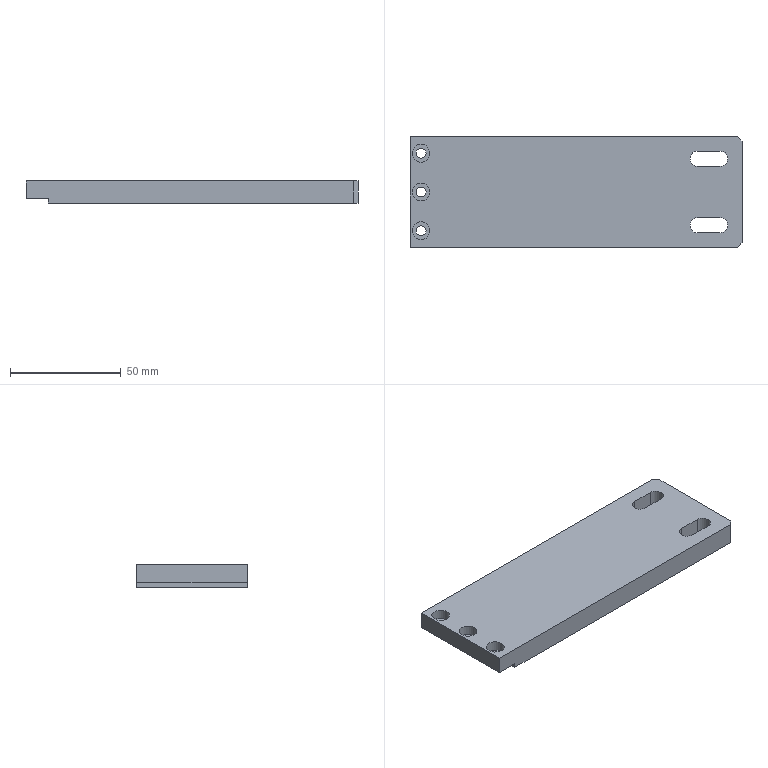Part | NX | 1 solid | 27 faces | box 150 x 50 x 10 mm | volume 70934 mm3 | plane 17 | cylinder 10 | commonest cylinder face diameters 7 x4 4.5 x3 8 x3
STEP:
#1=CARTESIAN_POINT('',(-75.,-25.,2.));
#2=VERTEX_POINT('',#1);
#3=CARTESIAN_POINT('',(-75.,25.,2.));
#4=VERTEX_POINT('',#3);
#5=CARTESIAN_POINT('',(-75.,-25.,2.));
#6=DIRECTION('',(0.,1.,0.));
#7=VECTOR('',#6,1000.);
#8=LINE('',#5,#7);
#9=EDGE_CURVE('',#2,#4,#8,.T.);
#10=ORIENTED_EDGE('',*,*,#9,.F.);
#11=CARTESIAN_POINT('',(-75.,-25.,10.));
#12=VERTEX_POINT('',#11);
#13=CARTESIAN_POINT('',(-75.,-25.,10.));
#14=DIRECTION('',(0.,0.,-1.));
#15=VECTOR('',#14,1000.);
#16=LINE('',#13,#15);
#17=EDGE_CURVE('',#12,#2,#16,.T.);
#18=ORIENTED_EDGE('',*,*,#17,.F.);
#19=CARTESIAN_POINT('',(-75.,25.,10.));
#20=VERTEX_POINT('',#19);
#21=CARTESIAN_POINT('',(-75.,-25.,10.));
#22=DIRECTION('',(0.,-1.,0.));
#23=VECTOR('',#22,1000.);
#24=LINE('',#21,#23);
#25=EDGE_CURVE('',#20,#12,#24,.T.);
#26=ORIENTED_EDGE('',*,*,#25,.F.);
#27=CARTESIAN_POINT('',(-75.,25.,10.));
#28=DIRECTION('',(0.,0.,-1.));
#29=VECTOR('',#28,1000.);
#30=LINE('',#27,#29);
#31=EDGE_CURVE('',#20,#4,#30,.T.);
#32=ORIENTED_EDGE('',*,*,#31,.T.);
#33=EDGE_LOOP('',(#10,#18,#26,#32));
#34=FACE_BOUND('',#33,.T.);
#35=CARTESIAN_POINT('',(-75.,-25.,10.));
#36=DIRECTION('',(1.,0.,0.));
#37=DIRECTION('',(0.,0.,-1.));
#38=AXIS2_PLACEMENT_3D('',#35,#36,#37);
#39=PLANE('',#38);
#40=ADVANCED_FACE('',(#34),#39,.F.);
#41=CARTESIAN_POINT('',(-67.75,-17.5,5.4));
#42=VERTEX_POINT('',#41);
#43=CARTESIAN_POINT('',(-70.,-17.5,5.4));
#44=DIRECTION('',(0.,0.,1.));
#45=DIRECTION('',(1.,0.,0.));
#46=AXIS2_PLACEMENT_3D('',#43,#44,#45);
#47=CIRCLE('',#46,2.25);
#48=EDGE_CURVE('',#42,#42,#47,.T.);
#49=ORIENTED_EDGE('',*,*,#48,.T.);
#50=EDGE_LOOP('',(#49));
#51=FACE_BOUND('',#50,.T.);
#52=CARTESIAN_POINT('',(-72.25,-17.5,2.));
#53=VERTEX_POINT('',#52);
#54=CARTESIAN_POINT('',(-70.,-17.5,2.));
#55=DIRECTION('',(0.,0.,-1.));
#56=DIRECTION('',(-1.,0.,0.));
#57=AXIS2_PLACEMENT_3D('',#54,#55,#56);
#58=CIRCLE('',#57,2.25);
#59=EDGE_CURVE('',#53,#53,#58,.F.);
#60=ORIENTED_EDGE('',*,*,#59,.F.);
#61=EDGE_LOOP('',(#60));
#62=FACE_BOUND('',#61,.T.);
#63=CARTESIAN_POINT('',(-70.,-17.5,10.));
#64=DIRECTION('',(0.,0.,1.));
#65=DIRECTION('',(1.,0.,0.));
#66=AXIS2_PLACEMENT_3D('',#63,#64,#65);
#67=CYLINDRICAL_SURFACE('',#66,2.25);
#68=ADVANCED_FACE('',(#51,#62),#67,.F.);
#69=CARTESIAN_POINT('',(-67.75,0.,5.4));
#70=VERTEX_POINT('',#69);
#71=CARTESIAN_POINT('',(-70.,0.,5.4));
#72=DIRECTION('',(0.,0.,1.));
#73=DIRECTION('',(1.,0.,0.));
#74=AXIS2_PLACEMENT_3D('',#71,#72,#73);
#75=CIRCLE('',#74,2.25);
#76=EDGE_CURVE('',#70,#70,#75,.T.);
#77=ORIENTED_EDGE('',*,*,#76,.T.);
#78=EDGE_LOOP('',(#77));
#79=FACE_BOUND('',#78,.T.);
#80=CARTESIAN_POINT('',(-72.25,0.,2.));
#81=VERTEX_POINT('',#80);
#82=CARTESIAN_POINT('',(-70.,0.,2.));
#83=DIRECTION('',(0.,0.,-1.));
#84=DIRECTION('',(-1.,0.,0.));
#85=AXIS2_PLACEMENT_3D('',#82,#83,#84);
#86=CIRCLE('',#85,2.25);
#87=EDGE_CURVE('',#81,#81,#86,.F.);
#88=ORIENTED_EDGE('',*,*,#87,.F.);
#89=EDGE_LOOP('',(#88));
#90=FACE_BOUND('',#89,.T.);
#91=CARTESIAN_POINT('',(-70.,0.,10.));
#92=DIRECTION('',(0.,0.,1.));
#93=DIRECTION('',(1.,0.,0.));
#94=AXIS2_PLACEMENT_3D('',#91,#92,#93);
#95=CYLINDRICAL_SURFACE('',#94,2.25);
#96=ADVANCED_FACE('',(#79,#90),#95,.F.);
#97=CARTESIAN_POINT('',(-67.75,17.5,5.4));
#98=VERTEX_POINT('',#97);
#99=CARTESIAN_POINT('',(-70.,17.5,5.4));
#100=DIRECTION('',(0.,0.,1.));
#101=DIRECTION('',(1.,0.,0.));
#102=AXIS2_PLACEMENT_3D('',#99,#100,#101);
#103=CIRCLE('',#102,2.25);
#104=EDGE_CURVE('',#98,#98,#103,.T.);
#105=ORIENTED_EDGE('',*,*,#104,.T.);
#106=EDGE_LOOP('',(#105));
#107=FACE_BOUND('',#106,.T.);
#108=CARTESIAN_POINT('',(-72.25,17.5,2.));
#109=VERTEX_POINT('',#108);
#110=CARTESIAN_POINT('',(-70.,17.5,2.));
#111=DIRECTION('',(0.,0.,-1.));
#112=DIRECTION('',(-1.,0.,0.));
#113=AXIS2_PLACEMENT_3D('',#110,#111,#112);
#114=CIRCLE('',#113,2.25);
#115=EDGE_CURVE('',#109,#109,#114,.F.);
#116=ORIENTED_EDGE('',*,*,#115,.F.);
#117=EDGE_LOOP('',(#116));
#118=FACE_BOUND('',#117,.T.);
#119=CARTESIAN_POINT('',(-70.,17.5,10.));
#120=DIRECTION('',(0.,0.,1.));
#121=DIRECTION('',(1.,0.,0.));
#122=AXIS2_PLACEMENT_3D('',#119,#120,#121);
#123=CYLINDRICAL_SURFACE('',#122,2.25);
#124=ADVANCED_FACE('',(#107,#118),#123,.F.);
#125=CARTESIAN_POINT('',(-65.,-25.,0.));
#126=VERTEX_POINT('',#125);
#127=CARTESIAN_POINT('',(73.,-25.,0.));
#128=VERTEX_POINT('',#127);
#129=CARTESIAN_POINT('',(75.,-25.,0.));
#130=DIRECTION('',(1.,0.,0.));
#131=VECTOR('',#130,1000.);
#132=LINE('',#129,#131);
#133=EDGE_CURVE('',#126,#128,#132,.T.);
#134=ORIENTED_EDGE('',*,*,#133,.T.);
#135=CARTESIAN_POINT('',(73.,-25.,10.));
#136=VERTEX_POINT('',#135);
#137=CARTESIAN_POINT('',(73.,-25.,10.));
#138=DIRECTION('',(0.,0.,1.));
#139=VECTOR('',#138,1000.);
#140=LINE('',#137,#139);
#141=EDGE_CURVE('',#128,#136,#140,.T.);
#142=ORIENTED_EDGE('',*,*,#141,.T.);
#143=CARTESIAN_POINT('',(75.,-25.,10.));
#144=DIRECTION('',(1.,0.,0.));
#145=VECTOR('',#144,1000.);
#146=LINE('',#143,#145);
#147=EDGE_CURVE('',#12,#136,#146,.T.);
#148=ORIENTED_EDGE('',*,*,#147,.F.);
#149=ORIENTED_EDGE('',*,*,#17,.T.);
#150=CARTESIAN_POINT('',(-65.,-25.,2.));
#151=VERTEX_POINT('',#150);
#152=CARTESIAN_POINT('',(-75.,-25.,2.));
#153=DIRECTION('',(-1.,0.,0.));
#154=VECTOR('',#153,1000.);
#155=LINE('',#152,#154);
#156=EDGE_CURVE('',#151,#2,#155,.T.);
#157=ORIENTED_EDGE('',*,*,#156,.F.);
#158=CARTESIAN_POINT('',(-65.,-25.,2.));
#159=DIRECTION('',(0.,0.,-1.));
#160=VECTOR('',#159,1000.);
#161=LINE('',#158,#160);
#162=EDGE_CURVE('',#151,#126,#161,.T.);
#163=ORIENTED_EDGE('',*,*,#162,.T.);
#164=EDGE_LOOP('',(#134,#142,#148,#149,#157,#163));
#165=FACE_BOUND('',#164,.T.);
#166=CARTESIAN_POINT('',(75.,-25.,10.));
#167=DIRECTION('',(0.,1.,0.));
#168=DIRECTION('',(-1.,0.,0.));
#169=AXIS2_PLACEMENT_3D('',#166,#167,#168);
#170=PLANE('',#169);
#171=ADVANCED_FACE('',(#165),#170,.F.);
#172=CARTESIAN_POINT('',(75.,-23.,10.));
#173=VERTEX_POINT('',#172);
#174=CARTESIAN_POINT('',(75.,23.,10.));
#175=VERTEX_POINT('',#174);
#176=CARTESIAN_POINT('',(75.,-25.,10.));
#177=DIRECTION('',(0.,1.,0.));
#178=VECTOR('',#177,1000.);
#179=LINE('',#176,#178);
#180=EDGE_CURVE('',#173,#175,#179,.T.);
#181=ORIENTED_EDGE('',*,*,#180,.F.);
#182=CARTESIAN_POINT('',(75.,-23.,0.));
#183=VERTEX_POINT('',#182);
#184=CARTESIAN_POINT('',(75.,-23.,10.));
#185=DIRECTION('',(0.,0.,-1.));
#186=VECTOR('',#185,1000.);
#187=LINE('',#184,#186);
#188=EDGE_CURVE('',#173,#183,#187,.T.);
#189=ORIENTED_EDGE('',*,*,#188,.T.);
#190=CARTESIAN_POINT('',(75.,23.,0.));
#191=VERTEX_POINT('',#190);
#192=CARTESIAN_POINT('',(75.,-25.,0.));
#193=DIRECTION('',(0.,1.,0.));
#194=VECTOR('',#193,1000.);
#195=LINE('',#192,#194);
#196=EDGE_CURVE('',#183,#191,#195,.T.);
#197=ORIENTED_EDGE('',*,*,#196,.T.);
#198=CARTESIAN_POINT('',(75.,23.,10.));
#199=DIRECTION('',(0.,0.,1.));
#200=VECTOR('',#199,1000.);
#201=LINE('',#198,#200);
#202=EDGE_CURVE('',#191,#175,#201,.T.);
#203=ORIENTED_EDGE('',*,*,#202,.T.);
#204=EDGE_LOOP('',(#181,#189,#197,#203));
#205=FACE_BOUND('',#204,.T.);
#206=CARTESIAN_POINT('',(75.,-25.,10.));
#207=DIRECTION('',(-1.,0.,0.));
#208=DIRECTION('',(0.,0.,1.));
#209=AXIS2_PLACEMENT_3D('',#206,#207,#208);
#210=PLANE('',#209);
#211=ADVANCED_FACE('',(#205),#210,.F.);
#212=CARTESIAN_POINT('',(73.,25.,10.));
#213=VERTEX_POINT('',#212);
#214=CARTESIAN_POINT('',(75.,25.,10.));
#215=DIRECTION('',(-1.,0.,0.));
#216=VECTOR('',#215,1000.);
#217=LINE('',#214,#216);
#218=EDGE_CURVE('',#213,#20,#217,.T.);
#219=ORIENTED_EDGE('',*,*,#218,.F.);
#220=CARTESIAN_POINT('',(73.,25.,0.));
#221=VERTEX_POINT('',#220);
#222=CARTESIAN_POINT('',(73.,25.,10.));
#223=DIRECTION('',(0.,0.,-1.));
#224=VECTOR('',#223,1000.);
#225=LINE('',#222,#224);
#226=EDGE_CURVE('',#213,#221,#225,.T.);
#227=ORIENTED_EDGE('',*,*,#226,.T.);
#228=CARTESIAN_POINT('',(-65.,25.,0.));
#229=VERTEX_POINT('',#228);
#230=CARTESIAN_POINT('',(75.,25.,0.));
#231=DIRECTION('',(-1.,0.,0.));
#232=VECTOR('',#231,1000.);
#233=LINE('',#230,#232);
#234=EDGE_CURVE('',#221,#229,#233,.T.);
#235=ORIENTED_EDGE('',*,*,#234,.T.);
#236=CARTESIAN_POINT('',(-65.,25.,2.));
#237=VERTEX_POINT('',#236);
#238=CARTESIAN_POINT('',(-65.,25.,2.));
#239=DIRECTION('',(0.,0.,-1.));
#240=VECTOR('',#239,1000.);
#241=LINE('',#238,#240);
#242=EDGE_CURVE('',#237,#229,#241,.T.);
#243=ORIENTED_EDGE('',*,*,#242,.F.);
#244=CARTESIAN_POINT('',(-75.,25.,2.));
#245=DIRECTION('',(1.,0.,0.));
#246=VECTOR('',#245,1000.);
#247=LINE('',#244,#246);
#248=EDGE_CURVE('',#4,#237,#247,.T.);
#249=ORIENTED_EDGE('',*,*,#248,.F.);
#250=ORIENTED_EDGE('',*,*,#31,.F.);
#251=EDGE_LOOP('',(#219,#227,#235,#243,#249,#250));
#252=FACE_BOUND('',#251,.T.);
#253=CARTESIAN_POINT('',(75.,25.,10.));
#254=DIRECTION('',(0.,-1.,0.));
#255=DIRECTION('',(1.,0.,0.));
#256=AXIS2_PLACEMENT_3D('',#253,#254,#255);
#257=PLANE('',#256);
#258=ADVANCED_FACE('',(#252),#257,.F.);
#259=CARTESIAN_POINT('',(55.,-11.5,10.));
#260=VERTEX_POINT('',#259);
#261=CARTESIAN_POINT('',(55.,-18.5,10.));
#262=VERTEX_POINT('',#261);
#263=CARTESIAN_POINT('',(55.,-15.,10.));
#264=DIRECTION('',(0.,0.,1.));
#265=DIRECTION('',(1.,0.,0.));
#266=AXIS2_PLACEMENT_3D('',#263,#264,#265);
#267=CIRCLE('',#266,3.5);
#268=EDGE_CURVE('',#260,#262,#267,.T.);
#269=ORIENTED_EDGE('',*,*,#268,.F.);
#270=CARTESIAN_POINT('',(65.,-11.5,10.));
#271=VERTEX_POINT('',#270);
#272=CARTESIAN_POINT('',(55.,-11.5,10.));
#273=DIRECTION('',(-1.,0.,0.));
#274=VECTOR('',#273,1000.);
#275=LINE('',#272,#274);
#276=EDGE_CURVE('',#271,#260,#275,.T.);
#277=ORIENTED_EDGE('',*,*,#276,.F.);
#278=CARTESIAN_POINT('',(65.,-18.5,10.));
#279=VERTEX_POINT('',#278);
#280=CARTESIAN_POINT('',(65.,-15.,10.));
#281=DIRECTION('',(0.,0.,1.));
#282=DIRECTION('',(1.,0.,0.));
#283=AXIS2_PLACEMENT_3D('',#280,#281,#282);
#284=CIRCLE('',#283,3.5);
#285=EDGE_CURVE('',#279,#271,#284,.T.);
#286=ORIENTED_EDGE('',*,*,#285,.F.);
#287=CARTESIAN_POINT('',(55.,-18.5,10.));
#288=DIRECTION('',(1.,0.,0.));
#289=VECTOR('',#288,1000.);
#290=LINE('',#287,#289);
#291=EDGE_CURVE('',#262,#279,#290,.T.);
#292=ORIENTED_EDGE('',*,*,#291,.F.);
#293=EDGE_LOOP('',(#269,#277,#286,#292));
#294=FACE_BOUND('',#293,.T.);
#295=CARTESIAN_POINT('',(55.,18.5,10.));
#296=VERTEX_POINT('',#295);
#297=CARTESIAN_POINT('',(55.,11.5,10.));
#298=VERTEX_POINT('',#297);
#299=CARTESIAN_POINT('',(55.,15.,10.));
#300=DIRECTION('',(0.,0.,1.));
#301=DIRECTION('',(1.,0.,0.));
#302=AXIS2_PLACEMENT_3D('',#299,#300,#301);
#303=CIRCLE('',#302,3.5);
#304=EDGE_CURVE('',#296,#298,#303,.T.);
#305=ORIENTED_EDGE('',*,*,#304,.F.);
#306=CARTESIAN_POINT('',(65.,18.5,10.));
#307=VERTEX_POINT('',#306);
#308=CARTESIAN_POINT('',(55.,18.5,10.));
#309=DIRECTION('',(-1.,0.,0.));
#310=VECTOR('',#309,1000.);
#311=LINE('',#308,#310);
#312=EDGE_CURVE('',#307,#296,#311,.T.);
#313=ORIENTED_EDGE('',*,*,#312,.F.);
#314=CARTESIAN_POINT('',(65.,11.5,10.));
#315=VERTEX_POINT('',#314);
#316=CARTESIAN_POINT('',(65.,15.,10.));
#317=DIRECTION('',(0.,0.,1.));
#318=DIRECTION('',(1.,0.,0.));
#319=AXIS2_PLACEMENT_3D('',#316,#317,#318);
#320=CIRCLE('',#319,3.5);
#321=EDGE_CURVE('',#315,#307,#320,.T.);
#322=ORIENTED_EDGE('',*,*,#321,.F.);
#323=CARTESIAN_POINT('',(55.,11.5,10.));
#324=DIRECTION('',(1.,0.,0.));
#325=VECTOR('',#324,1000.);
#326=LINE('',#323,#325);
#327=EDGE_CURVE('',#298,#315,#326,.T.);
#328=ORIENTED_EDGE('',*,*,#327,.F.);
#329=EDGE_LOOP('',(#305,#313,#322,#328));
#330=FACE_BOUND('',#329,.T.);
#331=CARTESIAN_POINT('',(-66.,17.5,10.));
#332=VERTEX_POINT('',#331);
#333=CARTESIAN_POINT('',(-70.,17.5,10.));
#334=DIRECTION('',(0.,0.,1.));
#335=DIRECTION('',(1.,0.,0.));
#336=AXIS2_PLACEMENT_3D('',#333,#334,#335);
#337=CIRCLE('',#336,4.);
#338=EDGE_CURVE('',#332,#332,#337,.T.);
#339=ORIENTED_EDGE('',*,*,#338,.F.);
#340=EDGE_LOOP('',(#339));
#341=FACE_BOUND('',#340,.T.);
#342=CARTESIAN_POINT('',(-66.,0.,10.));
#343=VERTEX_POINT('',#342);
#344=CARTESIAN_POINT('',(-70.,0.,10.));
#345=DIRECTION('',(0.,0.,1.));
#346=DIRECTION('',(1.,0.,0.));
#347=AXIS2_PLACEMENT_3D('',#344,#345,#346);
#348=CIRCLE('',#347,4.);
#349=EDGE_CURVE('',#343,#343,#348,.T.);
#350=ORIENTED_EDGE('',*,*,#349,.F.);
#351=EDGE_LOOP('',(#350));
#352=FACE_BOUND('',#351,.T.);
#353=CARTESIAN_POINT('',(-66.,-17.5,10.));
#354=VERTEX_POINT('',#353);
#355=CARTESIAN_POINT('',(-70.,-17.5,10.));
#356=DIRECTION('',(0.,0.,1.));
#357=DIRECTION('',(1.,0.,0.));
#358=AXIS2_PLACEMENT_3D('',#355,#356,#357);
#359=CIRCLE('',#358,4.);
#360=EDGE_CURVE('',#354,#354,#359,.T.);
#361=ORIENTED_EDGE('',*,*,#360,.F.);
#362=EDGE_LOOP('',(#361));
#363=FACE_BOUND('',#362,.T.);
#364=ORIENTED_EDGE('',*,*,#147,.T.);
#365=CARTESIAN_POINT('',(49.,-49.,10.));
#366=DIRECTION('',(-0.7071,-0.7071,0.));
#367=VECTOR('',#366,1000.);
#368=LINE('',#365,#367);
#369=EDGE_CURVE('',#136,#173,#368,.F.);
#370=ORIENTED_EDGE('',*,*,#369,.T.);
#371=ORIENTED_EDGE('',*,*,#180,.T.);
#372=CARTESIAN_POINT('',(49.,49.,10.));
#373=DIRECTION('',(0.7071,-0.7071,0.));
#374=VECTOR('',#373,1000.);
#375=LINE('',#372,#374);
#376=EDGE_CURVE('',#175,#213,#375,.F.);
#377=ORIENTED_EDGE('',*,*,#376,.T.);
#378=ORIENTED_EDGE('',*,*,#218,.T.);
#379=ORIENTED_EDGE('',*,*,#25,.T.);
#380=EDGE_LOOP('',(#364,#370,#371,#377,#378,#379));
#381=FACE_BOUND('',#380,.T.);
#382=CARTESIAN_POINT('',(0.,0.,10.));
#383=DIRECTION('',(0.,0.,1.));
#384=DIRECTION('',(1.,0.,0.));
#385=AXIS2_PLACEMENT_3D('',#382,#383,#384);
#386=PLANE('',#385);
#387=ADVANCED_FACE('',(#294,#330,#341,#352,#363,#381),#386,.T.);
#388=CARTESIAN_POINT('',(65.,-11.5,0.));
#389=VERTEX_POINT('',#388);
#390=CARTESIAN_POINT('',(55.,-11.5,0.));
#391=VERTEX_POINT('',#390);
#392=CARTESIAN_POINT('',(55.,-11.5,0.));
#393=DIRECTION('',(-1.,0.,0.));
#394=VECTOR('',#393,1000.);
#395=LINE('',#392,#394);
#396=EDGE_CURVE('',#389,#391,#395,.T.);
#397=ORIENTED_EDGE('',*,*,#396,.T.);
#398=CARTESIAN_POINT('',(55.,-18.5,0.));
#399=VERTEX_POINT('',#398);
#400=CARTESIAN_POINT('',(55.,-15.,0.));
#401=DIRECTION('',(0.,0.,1.));
#402=DIRECTION('',(1.,0.,0.));
#403=AXIS2_PLACEMENT_3D('',#400,#401,#402);
#404=CIRCLE('',#403,3.5);
#405=EDGE_CURVE('',#391,#399,#404,.T.);
#406=ORIENTED_EDGE('',*,*,#405,.T.);
#407=CARTESIAN_POINT('',(65.,-18.5,0.));
#408=VERTEX_POINT('',#407);
#409=CARTESIAN_POINT('',(55.,-18.5,0.));
#410=DIRECTION('',(1.,0.,0.));
#411=VECTOR('',#410,1000.);
#412=LINE('',#409,#411);
#413=EDGE_CURVE('',#399,#408,#412,.T.);
#414=ORIENTED_EDGE('',*,*,#413,.T.);
#415=CARTESIAN_POINT('',(65.,-15.,0.));
#416=DIRECTION('',(0.,0.,1.));
#417=DIRECTION('',(1.,0.,0.));
#418=AXIS2_PLACEMENT_3D('',#415,#416,#417);
#419=CIRCLE('',#418,3.5);
#420=EDGE_CURVE('',#408,#389,#419,.T.);
#421=ORIENTED_EDGE('',*,*,#420,.T.);
#422=EDGE_LOOP('',(#397,#406,#414,#421));
#423=FACE_BOUND('',#422,.T.);
#424=CARTESIAN_POINT('',(65.,18.5,0.));
#425=VERTEX_POINT('',#424);
#426=CARTESIAN_POINT('',(55.,18.5,0.));
#427=VERTEX_POINT('',#426);
#428=CARTESIAN_POINT('',(55.,18.5,0.));
#429=DIRECTION('',(-1.,0.,0.));
#430=VECTOR('',#429,1000.);
#431=LINE('',#428,#430);
#432=EDGE_CURVE('',#425,#427,#431,.T.);
#433=ORIENTED_EDGE('',*,*,#432,.T.);
#434=CARTESIAN_POINT('',(55.,11.5,0.));
#435=VERTEX_POINT('',#434);
#436=CARTESIAN_POINT('',(55.,15.,0.));
#437=DIRECTION('',(0.,0.,1.));
#438=DIRECTION('',(1.,0.,0.));
#439=AXIS2_PLACEMENT_3D('',#436,#437,#438);
#440=CIRCLE('',#439,3.5);
#441=EDGE_CURVE('',#427,#435,#440,.T.);
#442=ORIENTED_EDGE('',*,*,#441,.T.);
#443=CARTESIAN_POINT('',(65.,11.5,0.));
#444=VERTEX_POINT('',#443);
#445=CARTESIAN_POINT('',(55.,11.5,0.));
#446=DIRECTION('',(1.,0.,0.));
#447=VECTOR('',#446,1000.);
#448=LINE('',#445,#447);
#449=EDGE_CURVE('',#435,#444,#448,.T.);
#450=ORIENTED_EDGE('',*,*,#449,.T.);
#451=CARTESIAN_POINT('',(65.,15.,0.));
#452=DIRECTION('',(0.,0.,1.));
#453=DIRECTION('',(1.,0.,0.));
#454=AXIS2_PLACEMENT_3D('',#451,#452,#453);
#455=CIRCLE('',#454,3.5);
#456=EDGE_CURVE('',#444,#425,#455,.T.);
#457=ORIENTED_EDGE('',*,*,#456,.T.);
#458=EDGE_LOOP('',(#433,#442,#450,#457));
#459=FACE_BOUND('',#458,.T.);
#460=ORIENTED_EDGE('',*,*,#196,.F.);
#461=CARTESIAN_POINT('',(75.,-23.,0.));
#462=DIRECTION('',(0.7071,0.7071,0.));
#463=VECTOR('',#462,1000.);
#464=LINE('',#461,#463);
#465=EDGE_CURVE('',#183,#128,#464,.F.);
#466=ORIENTED_EDGE('',*,*,#465,.T.);
#467=ORIENTED_EDGE('',*,*,#133,.F.);
#468=CARTESIAN_POINT('',(-65.,-25.,0.));
#469=DIRECTION('',(0.,-1.,0.));
#470=VECTOR('',#469,1000.);
#471=LINE('',#468,#470);
#472=EDGE_CURVE('',#229,#126,#471,.T.);
#473=ORIENTED_EDGE('',*,*,#472,.F.);
#474=ORIENTED_EDGE('',*,*,#234,.F.);
#475=CARTESIAN_POINT('',(73.,25.,0.));
#476=DIRECTION('',(-0.7071,0.7071,0.));
#477=VECTOR('',#476,1000.);
#478=LINE('',#475,#477);
#479=EDGE_CURVE('',#221,#191,#478,.F.);
#480=ORIENTED_EDGE('',*,*,#479,.T.);
#481=EDGE_LOOP('',(#460,#466,#467,#473,#474,#480));
#482=FACE_BOUND('',#481,.T.);
#483=CARTESIAN_POINT('',(0.,0.,0.));
#484=DIRECTION('',(0.,0.,1.));
#485=DIRECTION('',(1.,0.,0.));
#486=AXIS2_PLACEMENT_3D('',#483,#484,#485);
#487=PLANE('',#486);
#488=ADVANCED_FACE('',(#423,#459,#482),#487,.F.);
#489=ORIENTED_EDGE('',*,*,#48,.F.);
#490=EDGE_LOOP('',(#489));
#491=FACE_BOUND('',#490,.T.);
#492=CARTESIAN_POINT('',(-66.,-17.5,5.4));
#493=VERTEX_POINT('',#492);
#494=CARTESIAN_POINT('',(-70.,-17.5,5.4));
#495=DIRECTION('',(0.,0.,1.));
#496=DIRECTION('',(1.,0.,0.));
#497=AXIS2_PLACEMENT_3D('',#494,#495,#496);
#498=CIRCLE('',#497,4.);
#499=EDGE_CURVE('',#493,#493,#498,.T.);
#500=ORIENTED_EDGE('',*,*,#499,.T.);
#501=EDGE_LOOP('',(#500));
#502=FACE_BOUND('',#501,.T.);
#503=CARTESIAN_POINT('',(-67.75,-17.5,5.4));
#504=DIRECTION('',(0.,0.,-1.));
#505=DIRECTION('',(-1.,0.,0.));
#506=AXIS2_PLACEMENT_3D('',#503,#504,#505);
#507=PLANE('',#506);
#508=ADVANCED_FACE('',(#491,#502),#507,.F.);
#509=ORIENTED_EDGE('',*,*,#499,.F.);
#510=EDGE_LOOP('',(#509));
#511=FACE_BOUND('',#510,.T.);
#512=ORIENTED_EDGE('',*,*,#360,.T.);
#513=EDGE_LOOP('',(#512));
#514=FACE_BOUND('',#513,.T.);
#515=CARTESIAN_POINT('',(-70.,-17.5,10.));
#516=DIRECTION('',(0.,0.,1.));
#517=DIRECTION('',(1.,0.,0.));
#518=AXIS2_PLACEMENT_3D('',#515,#516,#517);
#519=CYLINDRICAL_SURFACE('',#518,4.);
#520=ADVANCED_FACE('',(#511,#514),#519,.F.);
#521=ORIENTED_EDGE('',*,*,#76,.F.);
#522=EDGE_LOOP('',(#521));
#523=FACE_BOUND('',#522,.T.);
#524=CARTESIAN_POINT('',(-66.,0.,5.4));
#525=VERTEX_POINT('',#524);
#526=CARTESIAN_POINT('',(-70.,0.,5.4));
#527=DIRECTION('',(0.,0.,1.));
#528=DIRECTION('',(1.,0.,0.));
#529=AXIS2_PLACEMENT_3D('',#526,#527,#528);
#530=CIRCLE('',#529,4.);
#531=EDGE_CURVE('',#525,#525,#530,.T.);
#532=ORIENTED_EDGE('',*,*,#531,.T.);
#533=EDGE_LOOP('',(#532));
#534=FACE_BOUND('',#533,.T.);
#535=CARTESIAN_POINT('',(-67.75,0.,5.4));
#536=DIRECTION('',(0.,0.,-1.));
#537=DIRECTION('',(-1.,0.,0.));
#538=AXIS2_PLACEMENT_3D('',#535,#536,#537);
#539=PLANE('',#538);
#540=ADVANCED_FACE('',(#523,#534),#539,.F.);
#541=ORIENTED_EDGE('',*,*,#531,.F.);
#542=EDGE_LOOP('',(#541));
#543=FACE_BOUND('',#542,.T.);
#544=ORIENTED_EDGE('',*,*,#349,.T.);
#545=EDGE_LOOP('',(#544));
#546=FACE_BOUND('',#545,.T.);
#547=CARTESIAN_POINT('',(-70.,0.,10.));
#548=DIRECTION('',(0.,0.,1.));
#549=DIRECTION('',(1.,0.,0.));
#550=AXIS2_PLACEMENT_3D('',#547,#548,#549);
#551=CYLINDRICAL_SURFACE('',#550,4.);
#552=ADVANCED_FACE('',(#543,#546),#551,.F.);
#553=ORIENTED_EDGE('',*,*,#104,.F.);
#554=EDGE_LOOP('',(#553));
#555=FACE_BOUND('',#554,.T.);
#556=CARTESIAN_POINT('',(-66.,17.5,5.4));
#557=VERTEX_POINT('',#556);
#558=CARTESIAN_POINT('',(-70.,17.5,5.4));
#559=DIRECTION('',(0.,0.,1.));
#560=DIRECTION('',(1.,0.,0.));
#561=AXIS2_PLACEMENT_3D('',#558,#559,#560);
#562=CIRCLE('',#561,4.);
#563=EDGE_CURVE('',#557,#557,#562,.T.);
#564=ORIENTED_EDGE('',*,*,#563,.T.);
#565=EDGE_LOOP('',(#564));
#566=FACE_BOUND('',#565,.T.);
#567=CARTESIAN_POINT('',(-67.75,17.5,5.4));
#568=DIRECTION('',(0.,0.,-1.));
#569=DIRECTION('',(-1.,0.,0.));
#570=AXIS2_PLACEMENT_3D('',#567,#568,#569);
#571=PLANE('',#570);
#572=ADVANCED_FACE('',(#555,#566),#571,.F.);
#573=ORIENTED_EDGE('',*,*,#563,.F.);
#574=EDGE_LOOP('',(#573));
#575=FACE_BOUND('',#574,.T.);
#576=ORIENTED_EDGE('',*,*,#338,.T.);
#577=EDGE_LOOP('',(#576));
#578=FACE_BOUND('',#577,.T.);
#579=CARTESIAN_POINT('',(-70.,17.5,10.));
#580=DIRECTION('',(0.,0.,1.));
#581=DIRECTION('',(1.,0.,0.));
#582=AXIS2_PLACEMENT_3D('',#579,#580,#581);
#583=CYLINDRICAL_SURFACE('',#582,4.);
#584=ADVANCED_FACE('',(#575,#578),#583,.F.);
#585=ORIENTED_EDGE('',*,*,#304,.T.);
#586=CARTESIAN_POINT('',(55.,11.5,0.));
#587=DIRECTION('',(0.,0.,1.));
#588=VECTOR('',#587,1000.);
#589=LINE('',#586,#588);
#590=EDGE_CURVE('',#435,#298,#589,.T.);
#591=ORIENTED_EDGE('',*,*,#590,.F.);
#592=ORIENTED_EDGE('',*,*,#441,.F.);
#593=CARTESIAN_POINT('',(55.,18.5,0.));
#594=DIRECTION('',(0.,0.,1.));
#595=VECTOR('',#594,1000.);
#596=LINE('',#593,#595);
#597=EDGE_CURVE('',#427,#296,#596,.T.);
#598=ORIENTED_EDGE('',*,*,#597,.T.);
#599=EDGE_LOOP('',(#585,#591,#592,#598));
#600=FACE_BOUND('',#599,.T.);
#601=CARTESIAN_POINT('',(55.,15.,0.));
#602=DIRECTION('',(0.,0.,1.));
#603=DIRECTION('',(1.,0.,0.));
#604=AXIS2_PLACEMENT_3D('',#601,#602,#603);
#605=CYLINDRICAL_SURFACE('',#604,3.5);
#606=ADVANCED_FACE('',(#600),#605,.F.);
#607=ORIENTED_EDGE('',*,*,#312,.T.);
#608=ORIENTED_EDGE('',*,*,#597,.F.);
#609=ORIENTED_EDGE('',*,*,#432,.F.);
#610=CARTESIAN_POINT('',(65.,18.5,0.));
#611=DIRECTION('',(0.,0.,1.));
#612=VECTOR('',#611,1000.);
#613=LINE('',#610,#612);
#614=EDGE_CURVE('',#425,#307,#613,.T.);
#615=ORIENTED_EDGE('',*,*,#614,.T.);
#616=EDGE_LOOP('',(#607,#608,#609,#615));
#617=FACE_BOUND('',#616,.T.);
#618=CARTESIAN_POINT('',(55.,18.5,0.));
#619=DIRECTION('',(0.,1.,0.));
#620=DIRECTION('',(0.,0.,1.));
#621=AXIS2_PLACEMENT_3D('',#618,#619,#620);
#622=PLANE('',#621);
#623=ADVANCED_FACE('',(#617),#622,.F.);
#624=ORIENTED_EDGE('',*,*,#321,.T.);
#625=ORIENTED_EDGE('',*,*,#614,.F.);
#626=ORIENTED_EDGE('',*,*,#456,.F.);
#627=CARTESIAN_POINT('',(65.,11.5,0.));
#628=DIRECTION('',(0.,0.,1.));
#629=VECTOR('',#628,1000.);
#630=LINE('',#627,#629);
#631=EDGE_CURVE('',#444,#315,#630,.T.);
#632=ORIENTED_EDGE('',*,*,#631,.T.);
#633=EDGE_LOOP('',(#624,#625,#626,#632));
#634=FACE_BOUND('',#633,.T.);
#635=CARTESIAN_POINT('',(65.,15.,0.));
#636=DIRECTION('',(0.,0.,1.));
#637=DIRECTION('',(1.,0.,0.));
#638=AXIS2_PLACEMENT_3D('',#635,#636,#637);
#639=CYLINDRICAL_SURFACE('',#638,3.5);
#640=ADVANCED_FACE('',(#634),#639,.F.);
#641=ORIENTED_EDGE('',*,*,#327,.T.);
#642=ORIENTED_EDGE('',*,*,#631,.F.);
#643=ORIENTED_EDGE('',*,*,#449,.F.);
#644=ORIENTED_EDGE('',*,*,#590,.T.);
#645=EDGE_LOOP('',(#641,#642,#643,#644));
#646=FACE_BOUND('',#645,.T.);
#647=CARTESIAN_POINT('',(55.,11.5,0.));
#648=DIRECTION('',(0.,-1.,0.));
#649=DIRECTION('',(1.,0.,0.));
#650=AXIS2_PLACEMENT_3D('',#647,#648,#649);
#651=PLANE('',#650);
#652=ADVANCED_FACE('',(#646),#651,.F.);
#653=ORIENTED_EDGE('',*,*,#268,.T.);
#654=CARTESIAN_POINT('',(55.,-18.5,0.));
#655=DIRECTION('',(0.,0.,1.));
#656=VECTOR('',#655,1000.);
#657=LINE('',#654,#656);
#658=EDGE_CURVE('',#399,#262,#657,.T.);
#659=ORIENTED_EDGE('',*,*,#658,.F.);
#660=ORIENTED_EDGE('',*,*,#405,.F.);
#661=CARTESIAN_POINT('',(55.,-11.5,0.));
#662=DIRECTION('',(0.,0.,1.));
#663=VECTOR('',#662,1000.);
#664=LINE('',#661,#663);
#665=EDGE_CURVE('',#391,#260,#664,.T.);
#666=ORIENTED_EDGE('',*,*,#665,.T.);
#667=EDGE_LOOP('',(#653,#659,#660,#666));
#668=FACE_BOUND('',#667,.T.);
#669=CARTESIAN_POINT('',(55.,-15.,0.));
#670=DIRECTION('',(0.,0.,1.));
#671=DIRECTION('',(1.,0.,0.));
#672=AXIS2_PLACEMENT_3D('',#669,#670,#671);
#673=CYLINDRICAL_SURFACE('',#672,3.5);
#674=ADVANCED_FACE('',(#668),#673,.F.);
#675=ORIENTED_EDGE('',*,*,#276,.T.);
#676=ORIENTED_EDGE('',*,*,#665,.F.);
#677=ORIENTED_EDGE('',*,*,#396,.F.);
#678=CARTESIAN_POINT('',(65.,-11.5,0.));
#679=DIRECTION('',(0.,0.,1.));
#680=VECTOR('',#679,1000.);
#681=LINE('',#678,#680);
#682=EDGE_CURVE('',#389,#271,#681,.T.);
#683=ORIENTED_EDGE('',*,*,#682,.T.);
#684=EDGE_LOOP('',(#675,#676,#677,#683));
#685=FACE_BOUND('',#684,.T.);
#686=CARTESIAN_POINT('',(55.,-11.5,0.));
#687=DIRECTION('',(0.,1.,0.));
#688=DIRECTION('',(-1.,0.,0.));
#689=AXIS2_PLACEMENT_3D('',#686,#687,#688);
#690=PLANE('',#689);
#691=ADVANCED_FACE('',(#685),#690,.F.);
#692=ORIENTED_EDGE('',*,*,#285,.T.);
#693=ORIENTED_EDGE('',*,*,#682,.F.);
#694=ORIENTED_EDGE('',*,*,#420,.F.);
#695=CARTESIAN_POINT('',(65.,-18.5,0.));
#696=DIRECTION('',(0.,0.,1.));
#697=VECTOR('',#696,1000.);
#698=LINE('',#695,#697);
#699=EDGE_CURVE('',#408,#279,#698,.T.);
#700=ORIENTED_EDGE('',*,*,#699,.T.);
#701=EDGE_LOOP('',(#692,#693,#694,#700));
#702=FACE_BOUND('',#701,.T.);
#703=CARTESIAN_POINT('',(65.,-15.,0.));
#704=DIRECTION('',(0.,0.,1.));
#705=DIRECTION('',(1.,0.,0.));
#706=AXIS2_PLACEMENT_3D('',#703,#704,#705);
#707=CYLINDRICAL_SURFACE('',#706,3.5);
#708=ADVANCED_FACE('',(#702),#707,.F.);
#709=ORIENTED_EDGE('',*,*,#291,.T.);
#710=ORIENTED_EDGE('',*,*,#699,.F.);
#711=ORIENTED_EDGE('',*,*,#413,.F.);
#712=ORIENTED_EDGE('',*,*,#658,.T.);
#713=EDGE_LOOP('',(#709,#710,#711,#712));
#714=FACE_BOUND('',#713,.T.);
#715=CARTESIAN_POINT('',(55.,-18.5,0.));
#716=DIRECTION('',(0.,-1.,0.));
#717=DIRECTION('',(1.,0.,0.));
#718=AXIS2_PLACEMENT_3D('',#715,#716,#717);
#719=PLANE('',#718);
#720=ADVANCED_FACE('',(#714),#719,.F.);
#721=ORIENTED_EDGE('',*,*,#87,.T.);
#722=EDGE_LOOP('',(#721));
#723=FACE_BOUND('',#722,.T.);
#724=ORIENTED_EDGE('',*,*,#9,.T.);
#725=ORIENTED_EDGE('',*,*,#248,.T.);
#726=CARTESIAN_POINT('',(-65.,-25.,2.));
#727=DIRECTION('',(0.,-1.,0.));
#728=VECTOR('',#727,1000.);
#729=LINE('',#726,#728);
#730=EDGE_CURVE('',#237,#151,#729,.T.);
#731=ORIENTED_EDGE('',*,*,#730,.T.);
#732=ORIENTED_EDGE('',*,*,#156,.T.);
#733=EDGE_LOOP('',(#724,#725,#731,#732));
#734=FACE_BOUND('',#733,.T.);
#735=ORIENTED_EDGE('',*,*,#115,.T.);
#736=EDGE_LOOP('',(#735));
#737=FACE_BOUND('',#736,.T.);
#738=ORIENTED_EDGE('',*,*,#59,.T.);
#739=EDGE_LOOP('',(#738));
#740=FACE_BOUND('',#739,.T.);
#741=CARTESIAN_POINT('',(0.,0.,2.));
#742=DIRECTION('',(0.,0.,-1.));
#743=DIRECTION('',(-1.,0.,0.));
#744=AXIS2_PLACEMENT_3D('',#741,#742,#743);
#745=PLANE('',#744);
#746=ADVANCED_FACE('',(#723,#734,#737,#740),#745,.T.);
#747=ORIENTED_EDGE('',*,*,#472,.T.);
#748=ORIENTED_EDGE('',*,*,#162,.F.);
#749=ORIENTED_EDGE('',*,*,#730,.F.);
#750=ORIENTED_EDGE('',*,*,#242,.T.);
#751=EDGE_LOOP('',(#747,#748,#749,#750));
#752=FACE_BOUND('',#751,.T.);
#753=CARTESIAN_POINT('',(-65.,-25.,2.));
#754=DIRECTION('',(1.,0.,0.));
#755=DIRECTION('',(0.,0.,-1.));
#756=AXIS2_PLACEMENT_3D('',#753,#754,#755);
#757=PLANE('',#756);
#758=ADVANCED_FACE('',(#752),#757,.F.);
#759=ORIENTED_EDGE('',*,*,#369,.F.);
#760=ORIENTED_EDGE('',*,*,#141,.F.);
#761=ORIENTED_EDGE('',*,*,#465,.F.);
#762=ORIENTED_EDGE('',*,*,#188,.F.);
#763=EDGE_LOOP('',(#759,#760,#761,#762));
#764=FACE_BOUND('',#763,.T.);
#765=CARTESIAN_POINT('',(75.,-23.,10.));
#766=DIRECTION('',(-0.7071,0.7071,0.));
#767=DIRECTION('',(0.,0.,-1.));
#768=AXIS2_PLACEMENT_3D('',#765,#766,#767);
#769=PLANE('',#768);
#770=ADVANCED_FACE('',(#764),#769,.F.);
#771=ORIENTED_EDGE('',*,*,#376,.F.);
#772=ORIENTED_EDGE('',*,*,#202,.F.);
#773=ORIENTED_EDGE('',*,*,#479,.F.);
#774=ORIENTED_EDGE('',*,*,#226,.F.);
#775=EDGE_LOOP('',(#771,#772,#773,#774));
#776=FACE_BOUND('',#775,.T.);
#777=CARTESIAN_POINT('',(73.,25.,10.));
#778=DIRECTION('',(-0.7071,-0.7071,0.));
#779=DIRECTION('',(0.,0.,-1.));
#780=AXIS2_PLACEMENT_3D('',#777,#778,#779);
#781=PLANE('',#780);
#782=ADVANCED_FACE('',(#776),#781,.F.);
#783=CLOSED_SHELL('',(#40,#68,#96,#124,#171,#211,#258,#387,#488,#508,#520,#540,#552,#572,#584,#606,#623,#640,#652,#674,#691,#708,#720,#746,#758,#770,#782));
#784=MANIFOLD_SOLID_BREP('',#783);
#785=(LENGTH_UNIT()NAMED_UNIT(*)SI_UNIT(.MILLI.,.METRE.));
#786=UNCERTAINTY_MEASURE_WITH_UNIT(LENGTH_MEASURE(0.00001),#785,'','');
#787=(NAMED_UNIT(*)PLANE_ANGLE_UNIT()SI_UNIT($,.RADIAN.));
#788=(NAMED_UNIT(*)SI_UNIT($,.STERADIAN.)SOLID_ANGLE_UNIT());
#789=(GEOMETRIC_REPRESENTATION_CONTEXT(3)GLOBAL_UNCERTAINTY_ASSIGNED_CONTEXT((#786))GLOBAL_UNIT_ASSIGNED_CONTEXT((#785,#787,#788))REPRESENTATION_CONTEXT('',''));
#790=ADVANCED_BREP_SHAPE_REPRESENTATION('',(#784),#789);